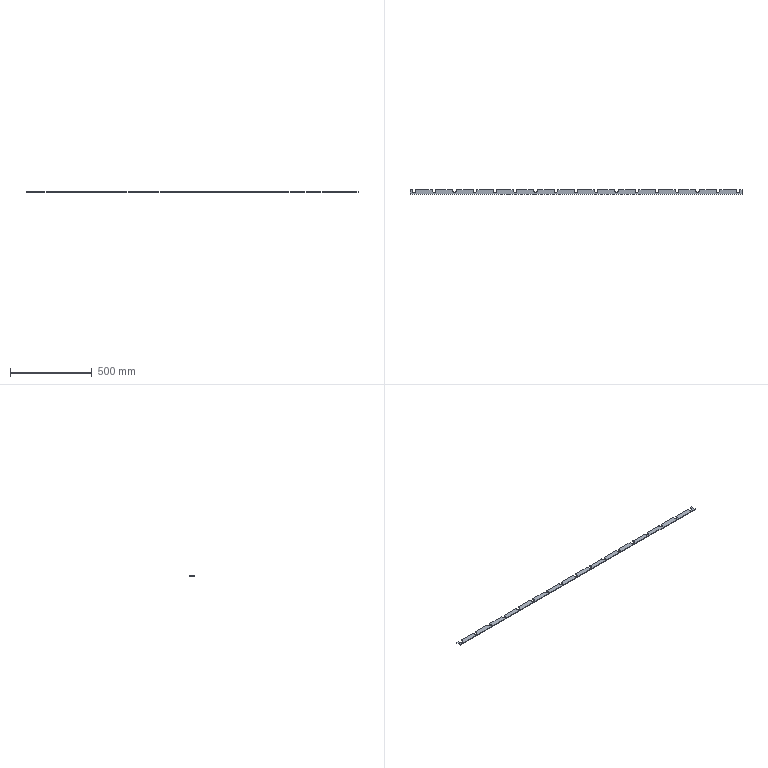Part | SolidWorks | features Extrusion 1, Fillet 1, ICE 1 | 1 solid | 108 faces | box 2030 x 30 x 4 mm | volume 219056 mm3 | plane 57 | cylinder 51 | commonest cylinder face diameters 6 x34 20 x17